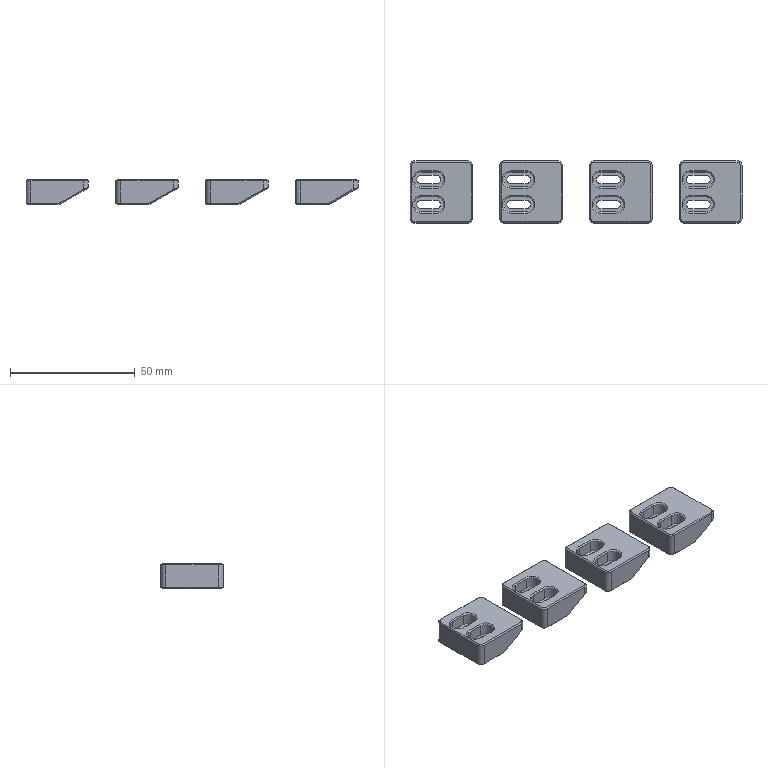NC program | NX | posted with a generic post | part box 133 x 25 x 10 mm
Lines 3494 to 3677 of 3677:
(PLANAR_MILL_COPY_COPY_COPY_COPY_COPY_COPY_1_COPY_1 , TOOL : D6A45)
N6980 T01 M6
N6982 G54
N6984 G17 G0 G90 X-48.134 Y7. S9500 M3
N6986 G43 Z30. H1
N6988 Z0.5
N6990 G94 G1 Z-1. F1250.
N6992 G3 X-49. Y7.5 R1.
N6994 G1 X-52.
N6996 G3 X-54.5 Y5. R2.5
N6998 X-52. Y2.5 R2.5
N7000 G1 X-46.
N7002 G3 X-43.5 Y5. R2.5
N7004 X-46. Y7.5 R2.5
N7006 G1 X-49.
N7008 G3 X-49.866 Y7. R1.
N7010 G1 Z0.5
N7012 G0 Z30.
N7014 X-54.866 Y13.5
N7016 Z0.5
N7018 G1 Z-1.
N7020 G3 X-54. Y13. R1.
N7022 G1 X-43.5
N7024 G2 X-41. Y10.5 R2.5
N7026 G1 Y-10.5
N7028 G2 X-43.5 Y-13. R2.5
N7030 G1 X-64.5
N7032 G2 X-67. Y-10.5 R2.5
N7034 G1 Y10.5
N7036 G2 X-64.5 Y13. R2.5
N7038 G1 X-54.
N7040 G3 X-53.134 Y13.5 R1.
N7042 G1 Z0.5
N7044 G0 Z30.
N7046 X-49.866 Y-7.
N7048 Z0.5
N7050 G1 Z-1.
N7052 G3 X-49. Y-7.5 R1.
N7054 G1 X-46.
N7056 G3 X-43.5 Y-5. R2.5
N7058 X-46. Y-2.5 R2.5
N7060 G1 X-52.
N7062 G3 X-54.5 Y-5. R2.5
N7064 X-52. Y-7.5 R2.5
N7066 G1 X-49.
N7068 G3 X-48.134 Y-7. R1.
N7070 G1 Z0.5
N7072 G0 Z30.
N7074 X-17.134 Y-13.5
N7076 Z0.5
N7078 G1 Z-1.
N7080 G3 X-18. Y-13. R1.
N7082 G1 X-28.5
N7084 G2 X-31. Y-10.5 R2.5
N7086 G1 Y10.5
N7088 G2 X-28.5 Y13. R2.5
N7090 G1 X-7.5
N7092 G2 X-5. Y10.5 R2.5
N7094 G1 Y-10.5
N7096 G2 X-7.5 Y-13. R2.5
N7098 G1 X-18.
N7100 G3 X-18.866 Y-13.5 R1.
N7102 G1 Z0.5
N7104 G0 Z30.
N7106 X-13.866 Y-7.
N7108 Z0.5
N7110 G1 Z-1.
N7112 G3 X-13. Y-7.5 R1.
N7114 G1 X-10.
N7116 G3 X-7.5 Y-5. R2.5
N7118 X-10. Y-2.5 R2.5
N7120 G1 X-16.
N7122 G3 X-18.5 Y-5. R2.5
N7124 X-16. Y-7.5 R2.5
N7126 G1 X-13.
N7128 G3 X-12.134 Y-7. R1.
N7130 G1 Z0.5
N7132 G0 Z30.
N7134 Y7.
N7136 Z0.5
N7138 G1 Z-1.
N7140 G3 X-13. Y7.5 R1.
N7142 G1 X-16.
N7144 G3 X-18.5 Y5. R2.5
N7146 X-16. Y2.5 R2.5
N7148 G1 X-10.
N7150 G3 X-7.5 Y5. R2.5
N7152 X-10. Y7.5 R2.5
N7154 G1 X-13.
N7156 G3 X-13.866 Y7. R1.
N7158 G1 Z0.5
N7160 G0 Z30.
N7162 X17.134 Y13.5
N7164 Z0.5
N7166 G1 Z-1.
N7168 G3 X18. Y13. R1.
N7170 G1 X28.5
N7172 G2 X31. Y10.5 R2.5
N7174 G1 Y-10.5
N7176 G2 X28.5 Y-13. R2.5
N7178 G1 X7.5
N7180 G2 X5. Y-10.5 R2.5
N7182 G1 Y10.5
N7184 G2 X7.5 Y13. R2.5
N7186 G1 X18.
N7188 G3 X18.866 Y13.5 R1.
N7190 G1 Z0.5
N7192 G0 Z30.
N7194 X23.866 Y7.
N7196 Z0.5
N7198 G1 Z-1.
N7200 G3 X23. Y7.5 R1.
N7202 G1 X20.
N7204 G3 X17.5 Y5. R2.5
N7206 X20. Y2.5 R2.5
N7208 G1 X26.
N7210 G3 X28.5 Y5. R2.5
N7212 X26. Y7.5 R2.5
N7214 G1 X23.
N7216 G3 X22.134 Y7. R1.
N7218 G1 Z0.5
N7220 G0 Z30.
N7222 Y-7.
N7224 Z0.5
N7226 G1 Z-1.
N7228 G3 X23. Y-7.5 R1.
N7230 G1 X26.
N7232 G3 X28.5 Y-5. R2.5
N7234 X26. Y-2.5 R2.5
N7236 G1 X20.
N7238 G3 X17.5 Y-5. R2.5
N7240 X20. Y-7.5 R2.5
N7242 G1 X23.
N7244 G3 X23.866 Y-7. R1.
N7246 G1 Z0.5
N7248 G0 Z30.
N7250 X54.866 Y-13.5
N7252 Z0.5
N7254 G1 Z-1.
N7256 G3 X54. Y-13. R1.
N7258 G1 X43.5
N7260 G2 X41. Y-10.5 R2.5
N7262 G1 Y10.5
N7264 G2 X43.5 Y13. R2.5
N7266 G1 X64.5
N7268 G2 X67. Y10.5 R2.5
N7270 G1 Y-10.5
N7272 G2 X64.5 Y-13. R2.5
N7274 G1 X54.
N7276 G3 X53.134 Y-13.5 R1.
N7278 G1 Z0.5
N7280 G0 Z30.
N7282 X58.134 Y-7.
N7284 Z0.5
N7286 G1 Z-1.
N7288 G3 X59. Y-7.5 R1.
N7290 G1 X62.
N7292 G3 X64.5 Y-5. R2.5
N7294 X62. Y-2.5 R2.5
N7296 G1 X56.
N7298 G3 X53.5 Y-5. R2.5
N7300 X56. Y-7.5 R2.5
N7302 G1 X59.
N7304 G3 X59.866 Y-7. R1.
N7306 G1 Z0.5
N7308 G0 Z30.
N7310 X58.134 Y3.
N7312 Z0.5
N7314 G1 Z-1.
N7316 G3 X59. Y2.5 R1.
N7318 G1 X62.
N7320 G3 X64.5 Y5. R2.5
N7322 X62. Y7.5 R2.5
N7324 G1 X56.
N7326 G3 X53.5 Y5. R2.5
N7328 X56. Y2.5 R2.5
N7330 G1 X59.
N7332 G3 X59.866 Y3. R1.
N7334 G1 Z0.5
N7336 G0 Z30.
N7338 M5
N7340 M2